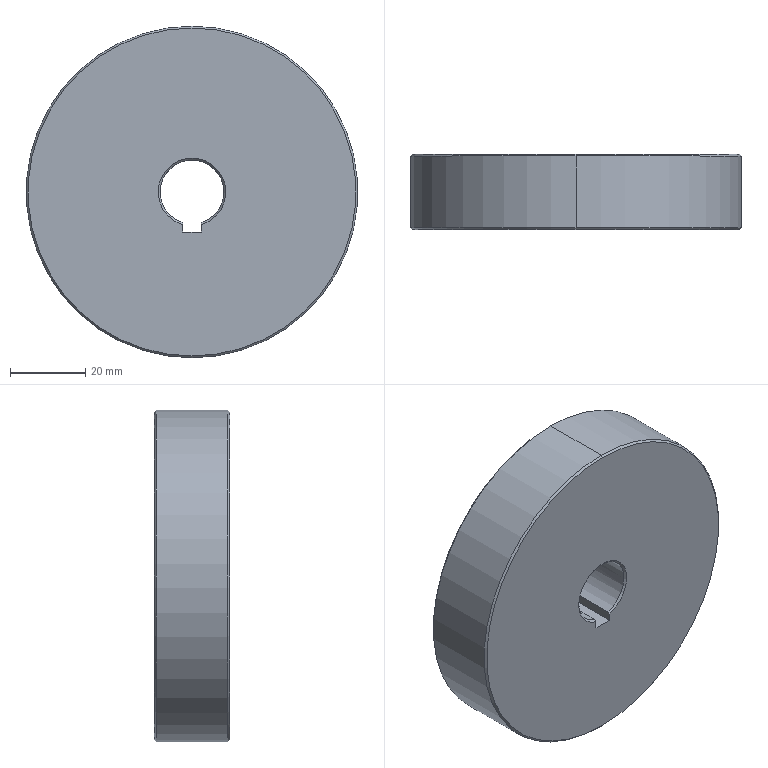Part | STEP file | Cuon T phu H01_6 | 1 solid | 15 faces | box 88 x 20 x 88 mm | volume 116797 mm3 | cone 7 | plane 5 | cylinder 3 | commonest cylinder face diameters 88 x2 17 x1
STEP:
#1=CARTESIAN_POINT('',(0.,0.,0.));
#2=DIRECTION('',(0.,0.,1.));
#3=DIRECTION('',(1.,0.,0.));
#4=AXIS2_PLACEMENT_3D('',#1,#2,#3);
#5=CARTESIAN_POINT('',(0.,20.,43.5));
#6=VERTEX_POINT('',#5);
#7=CARTESIAN_POINT('',(0.,20.,-43.5));
#8=VERTEX_POINT('',#7);
#9=CARTESIAN_POINT('',(0.,20.,0.));
#10=DIRECTION('',(0.,1.,0.));
#11=DIRECTION('',(0.,0.,1.));
#12=AXIS2_PLACEMENT_3D('',#9,#10,#11);
#13=CIRCLE('',#12,43.5);
#14=CARTESIAN_POINT('',(0.,20.,0.));
#15=DIRECTION('',(0.,-1.,0.));
#16=DIRECTION('',(0.,0.,-1.));
#17=AXIS2_PLACEMENT_3D('',#14,#15,#16);
#18=CONICAL_SURFACE('',#17,43.5,0.7854);
#19=CARTESIAN_POINT('',(3.142,0.));
#20=DIRECTION('',(-1.,0.));
#21=VECTOR('',#20,1.);
#22=LINE('',#19,#21);
#23=(GEOMETRIC_REPRESENTATION_CONTEXT(2)PARAMETRIC_REPRESENTATION_CONTEXT()REPRESENTATION_CONTEXT('',''));
#24=DEFINITIONAL_REPRESENTATION('',(#22),#23);
#25=PCURVE('',#18,#24);
#26=CARTESIAN_POINT('',(0.,20.,0.));
#27=DIRECTION('',(0.,1.,0.));
#28=DIRECTION('',(0.,0.,1.));
#29=AXIS2_PLACEMENT_3D('',#26,#27,#28);
#30=PLANE('',#29);
#31=CARTESIAN_POINT('',(0.,0.));
#32=DIRECTION('',(1.,0.));
#33=AXIS2_PLACEMENT_2D('',#31,#32);
#34=CIRCLE('',#33,43.5);
#35=(GEOMETRIC_REPRESENTATION_CONTEXT(2)PARAMETRIC_REPRESENTATION_CONTEXT()REPRESENTATION_CONTEXT('',''));
#36=DEFINITIONAL_REPRESENTATION('',(#34),#35);
#37=PCURVE('',#30,#36);
#38=SURFACE_CURVE('',#13,(#25,#37),.PCURVE_S1.);
#39=EDGE_CURVE('',#6,#8,#38,.T.);
#40=ORIENTED_EDGE('',*,*,#39,.F.);
#41=CARTESIAN_POINT('',(0.,19.5,44.));
#42=VERTEX_POINT('',#41);
#43=CARTESIAN_POINT('',(0.,20.,43.5));
#44=DIRECTION('',(0.,-0.7071,0.7071));
#45=VECTOR('',#44,1.);
#46=LINE('',#43,#45);
#47=CARTESIAN_POINT('',(3.142,0.));
#48=DIRECTION('',(0.,1.));
#49=VECTOR('',#48,1.);
#50=LINE('',#47,#49);
#51=(GEOMETRIC_REPRESENTATION_CONTEXT(2)PARAMETRIC_REPRESENTATION_CONTEXT()REPRESENTATION_CONTEXT('',''));
#52=DEFINITIONAL_REPRESENTATION('',(#50),#51);
#53=PCURVE('',#18,#52);
#54=CARTESIAN_POINT('',(0.,20.,0.));
#55=DIRECTION('',(0.,-1.,0.));
#56=DIRECTION('',(0.,0.,-1.));
#57=AXIS2_PLACEMENT_3D('',#54,#55,#56);
#58=CONICAL_SURFACE('',#57,43.5,0.7854);
#59=CARTESIAN_POINT('',(3.142,0.));
#60=DIRECTION('',(0.,1.));
#61=VECTOR('',#60,1.);
#62=LINE('',#59,#61);
#63=(GEOMETRIC_REPRESENTATION_CONTEXT(2)PARAMETRIC_REPRESENTATION_CONTEXT()REPRESENTATION_CONTEXT('',''));
#64=DEFINITIONAL_REPRESENTATION('',(#62),#63);
#65=PCURVE('',#58,#64);
#66=SURFACE_CURVE('',#46,(#53,#65),.PCURVE_S1.);
#67=EDGE_CURVE('',#6,#42,#66,.T.);
#68=ORIENTED_EDGE('',*,*,#67,.T.);
#69=CARTESIAN_POINT('',(0.,19.5,-44.));
#70=VERTEX_POINT('',#69);
#71=CARTESIAN_POINT('',(0.,19.5,0.));
#72=DIRECTION('',(0.,-1.,0.));
#73=DIRECTION('',(0.,0.,1.));
#74=AXIS2_PLACEMENT_3D('',#71,#72,#73);
#75=CIRCLE('',#74,44.);
#76=CARTESIAN_POINT('',(-3.142,0.5));
#77=DIRECTION('',(1.,0.));
#78=VECTOR('',#77,1.);
#79=LINE('',#76,#78);
#80=(GEOMETRIC_REPRESENTATION_CONTEXT(2)PARAMETRIC_REPRESENTATION_CONTEXT()REPRESENTATION_CONTEXT('',''));
#81=DEFINITIONAL_REPRESENTATION('',(#79),#80);
#82=PCURVE('',#18,#81);
#83=CARTESIAN_POINT('',(0.,20.,0.));
#84=DIRECTION('',(0.,-1.,0.));
#85=DIRECTION('',(0.,0.,-1.));
#86=AXIS2_PLACEMENT_3D('',#83,#84,#85);
#87=CYLINDRICAL_SURFACE('',#86,44.);
#88=CARTESIAN_POINT('',(-3.142,0.5));
#89=DIRECTION('',(1.,0.));
#90=VECTOR('',#89,1.);
#91=LINE('',#88,#90);
#92=(GEOMETRIC_REPRESENTATION_CONTEXT(2)PARAMETRIC_REPRESENTATION_CONTEXT()REPRESENTATION_CONTEXT('',''));
#93=DEFINITIONAL_REPRESENTATION('',(#91),#92);
#94=PCURVE('',#87,#93);
#95=SURFACE_CURVE('',#75,(#82,#94),.PCURVE_S1.);
#96=EDGE_CURVE('',#70,#42,#95,.T.);
#97=ORIENTED_EDGE('',*,*,#96,.F.);
#98=CARTESIAN_POINT('',(0.,20.,-43.5));
#99=DIRECTION('',(0.,-0.7071,-0.7071));
#100=VECTOR('',#99,1.);
#101=LINE('',#98,#100);
#102=CARTESIAN_POINT('',(0.,0.));
#103=DIRECTION('',(0.,1.));
#104=VECTOR('',#103,1.);
#105=LINE('',#102,#104);
#106=(GEOMETRIC_REPRESENTATION_CONTEXT(2)PARAMETRIC_REPRESENTATION_CONTEXT()REPRESENTATION_CONTEXT('',''));
#107=DEFINITIONAL_REPRESENTATION('',(#105),#106);
#108=PCURVE('',#18,#107);
#109=CARTESIAN_POINT('',(6.283,0.));
#110=DIRECTION('',(0.,1.));
#111=VECTOR('',#110,1.);
#112=LINE('',#109,#111);
#113=(GEOMETRIC_REPRESENTATION_CONTEXT(2)PARAMETRIC_REPRESENTATION_CONTEXT()REPRESENTATION_CONTEXT('',''));
#114=DEFINITIONAL_REPRESENTATION('',(#112),#113);
#115=PCURVE('',#58,#114);
#116=SURFACE_CURVE('',#101,(#108,#115),.PCURVE_S1.);
#117=EDGE_CURVE('',#8,#70,#116,.T.);
#118=ORIENTED_EDGE('',*,*,#117,.F.);
#119=EDGE_LOOP('',(#40,#68,#97,#118));
#120=FACE_BOUND('',#119,.T.);
#121=ADVANCED_FACE('',(#120),#18,.T.);
#122=CARTESIAN_POINT('',(0.,0.,-43.5));
#123=VERTEX_POINT('',#122);
#124=CARTESIAN_POINT('',(0.,0.,43.5));
#125=VERTEX_POINT('',#124);
#126=CARTESIAN_POINT('',(0.,0.,0.));
#127=DIRECTION('',(0.,-1.,0.));
#128=DIRECTION('',(0.,0.,1.));
#129=AXIS2_PLACEMENT_3D('',#126,#127,#128);
#130=CIRCLE('',#129,43.5);
#131=CARTESIAN_POINT('',(0.,0.5,0.));
#132=DIRECTION('',(0.,1.,0.));
#133=DIRECTION('',(0.,0.,1.));
#134=AXIS2_PLACEMENT_3D('',#131,#132,#133);
#135=CONICAL_SURFACE('',#134,44.,0.7854);
#136=CARTESIAN_POINT('',(6.283,-0.5));
#137=DIRECTION('',(-1.,0.));
#138=VECTOR('',#137,1.);
#139=LINE('',#136,#138);
#140=(GEOMETRIC_REPRESENTATION_CONTEXT(2)PARAMETRIC_REPRESENTATION_CONTEXT()REPRESENTATION_CONTEXT('',''));
#141=DEFINITIONAL_REPRESENTATION('',(#139),#140);
#142=PCURVE('',#135,#141);
#143=CARTESIAN_POINT('',(0.,0.,0.));
#144=DIRECTION('',(0.,1.,0.));
#145=DIRECTION('',(0.,0.,1.));
#146=AXIS2_PLACEMENT_3D('',#143,#144,#145);
#147=PLANE('',#146);
#148=CARTESIAN_POINT('',(43.5,0.));
#149=CARTESIAN_POINT('',(43.5,-75.344));
#150=CARTESIAN_POINT('',(-21.75,-37.672));
#151=CARTESIAN_POINT('',(-87.,0.));
#152=CARTESIAN_POINT('',(-21.75,37.672));
#153=CARTESIAN_POINT('',(43.5,75.344));
#154=CARTESIAN_POINT('',(43.5,0.));
#155=(BOUNDED_CURVE()B_SPLINE_CURVE(2,(#148,#149,#150,#151,#152,#153,#154),.UNSPECIFIED.,.T.,.F.)B_SPLINE_CURVE_WITH_KNOTS((1,2,2,2,2,1),(-2.094,0.,2.094,4.189,6.283,8.378),.UNSPECIFIED.)CURVE()GEOMETRIC_REPRESENTATION_ITEM()RATIONAL_B_SPLINE_CURVE((1.,0.5,1.,0.5,1.,0.5,1.))REPRESENTATION_ITEM(''));
#156=(GEOMETRIC_REPRESENTATION_CONTEXT(2)PARAMETRIC_REPRESENTATION_CONTEXT()REPRESENTATION_CONTEXT('',''));
#157=DEFINITIONAL_REPRESENTATION('',(#155),#156);
#158=PCURVE('',#147,#157);
#159=SURFACE_CURVE('',#130,(#142,#158),.PCURVE_S1.);
#160=EDGE_CURVE('',#123,#125,#159,.T.);
#161=ORIENTED_EDGE('',*,*,#160,.F.);
#162=CARTESIAN_POINT('',(0.,0.5,-44.));
#163=VERTEX_POINT('',#162);
#164=CARTESIAN_POINT('',(0.,0.5,-44.));
#165=DIRECTION('',(0.,0.7071,-0.7071));
#166=VECTOR('',#165,1.);
#167=LINE('',#164,#166);
#168=CARTESIAN_POINT('',(3.142,0.));
#169=DIRECTION('',(0.,1.));
#170=VECTOR('',#169,1.);
#171=LINE('',#168,#170);
#172=(GEOMETRIC_REPRESENTATION_CONTEXT(2)PARAMETRIC_REPRESENTATION_CONTEXT()REPRESENTATION_CONTEXT('',''));
#173=DEFINITIONAL_REPRESENTATION('',(#171),#172);
#174=PCURVE('',#135,#173);
#175=CARTESIAN_POINT('',(0.,0.5,0.));
#176=DIRECTION('',(0.,1.,0.));
#177=DIRECTION('',(0.,0.,1.));
#178=AXIS2_PLACEMENT_3D('',#175,#176,#177);
#179=CONICAL_SURFACE('',#178,44.,0.7854);
#180=CARTESIAN_POINT('',(3.142,0.));
#181=DIRECTION('',(0.,1.));
#182=VECTOR('',#181,1.);
#183=LINE('',#180,#182);
#184=(GEOMETRIC_REPRESENTATION_CONTEXT(2)PARAMETRIC_REPRESENTATION_CONTEXT()REPRESENTATION_CONTEXT('',''));
#185=DEFINITIONAL_REPRESENTATION('',(#183),#184);
#186=PCURVE('',#179,#185);
#187=SURFACE_CURVE('',#167,(#174,#186),.PCURVE_S1.);
#188=EDGE_CURVE('',#123,#163,#187,.T.);
#189=ORIENTED_EDGE('',*,*,#188,.T.);
#190=CARTESIAN_POINT('',(0.,0.5,44.));
#191=VERTEX_POINT('',#190);
#192=CARTESIAN_POINT('',(0.,0.5,0.));
#193=DIRECTION('',(0.,1.,0.));
#194=DIRECTION('',(0.,0.,1.));
#195=AXIS2_PLACEMENT_3D('',#192,#193,#194);
#196=CIRCLE('',#195,44.);
#197=CARTESIAN_POINT('',(0.,0.));
#198=DIRECTION('',(1.,0.));
#199=VECTOR('',#198,1.);
#200=LINE('',#197,#199);
#201=(GEOMETRIC_REPRESENTATION_CONTEXT(2)PARAMETRIC_REPRESENTATION_CONTEXT()REPRESENTATION_CONTEXT('',''));
#202=DEFINITIONAL_REPRESENTATION('',(#200),#201);
#203=PCURVE('',#135,#202);
#204=CARTESIAN_POINT('',(3.142,19.5));
#205=DIRECTION('',(-1.,0.));
#206=VECTOR('',#205,1.);
#207=LINE('',#204,#206);
#208=(GEOMETRIC_REPRESENTATION_CONTEXT(2)PARAMETRIC_REPRESENTATION_CONTEXT()REPRESENTATION_CONTEXT('',''));
#209=DEFINITIONAL_REPRESENTATION('',(#207),#208);
#210=PCURVE('',#87,#209);
#211=SURFACE_CURVE('',#196,(#203,#210),.PCURVE_S1.);
#212=EDGE_CURVE('',#191,#163,#211,.T.);
#213=ORIENTED_EDGE('',*,*,#212,.F.);
#214=CARTESIAN_POINT('',(0.,0.5,44.));
#215=DIRECTION('',(0.,0.7071,0.7071));
#216=VECTOR('',#215,1.);
#217=LINE('',#214,#216);
#218=CARTESIAN_POINT('',(0.,0.));
#219=DIRECTION('',(0.,1.));
#220=VECTOR('',#219,1.);
#221=LINE('',#218,#220);
#222=(GEOMETRIC_REPRESENTATION_CONTEXT(2)PARAMETRIC_REPRESENTATION_CONTEXT()REPRESENTATION_CONTEXT('',''));
#223=DEFINITIONAL_REPRESENTATION('',(#221),#222);
#224=PCURVE('',#135,#223);
#225=CARTESIAN_POINT('',(6.283,0.));
#226=DIRECTION('',(0.,1.));
#227=VECTOR('',#226,1.);
#228=LINE('',#225,#227);
#229=(GEOMETRIC_REPRESENTATION_CONTEXT(2)PARAMETRIC_REPRESENTATION_CONTEXT()REPRESENTATION_CONTEXT('',''));
#230=DEFINITIONAL_REPRESENTATION('',(#228),#229);
#231=PCURVE('',#179,#230);
#232=SURFACE_CURVE('',#217,(#224,#231),.PCURVE_S1.);
#233=EDGE_CURVE('',#125,#191,#232,.T.);
#234=ORIENTED_EDGE('',*,*,#233,.F.);
#235=EDGE_LOOP('',(#161,#189,#213,#234));
#236=FACE_BOUND('',#235,.T.);
#237=ADVANCED_FACE('',(#236),#135,.T.);
#238=CARTESIAN_POINT('',(2.5,19.5,-8.124));
#239=VERTEX_POINT('',#238);
#240=CARTESIAN_POINT('',(2.5,20.,-8.646));
#241=VERTEX_POINT('',#240);
#242=CARTESIAN_POINT('',(2.5,19.5,-8.124));
#243=CARTESIAN_POINT('',(2.5,19.666,-8.298));
#244=CARTESIAN_POINT('',(2.5,19.833,-8.472));
#245=CARTESIAN_POINT('',(2.5,20.,-8.646));
#246=B_SPLINE_CURVE_WITH_KNOTS('',3,(#242,#243,#244,#245),.UNSPECIFIED.,.F.,.F.,(4,4),(0.,0.0007227),.PIECEWISE_BEZIER_KNOTS.);
#247=CARTESIAN_POINT('',(0.,19.5,0.));
#248=DIRECTION('',(0.,1.,0.));
#249=DIRECTION('',(0.,0.,1.));
#250=AXIS2_PLACEMENT_3D('',#247,#248,#249);
#251=CONICAL_SURFACE('',#250,8.5,0.7854);
#252=CARTESIAN_POINT('',(2.843,0.));
#253=CARTESIAN_POINT('',(2.843,0.007565));
#254=CARTESIAN_POINT('',(2.844,0.0227));
#255=CARTESIAN_POINT('',(2.845,0.0454));
#256=CARTESIAN_POINT('',(2.846,0.0681));
#257=CARTESIAN_POINT('',(2.846,0.09081));
#258=CARTESIAN_POINT('',(2.847,0.1135));
#259=CARTESIAN_POINT('',(2.848,0.1362));
#260=CARTESIAN_POINT('',(2.849,0.1589));
#261=CARTESIAN_POINT('',(2.849,0.1817));
#262=CARTESIAN_POINT('',(2.85,0.2044));
#263=CARTESIAN_POINT('',(2.851,0.2271));
#264=CARTESIAN_POINT('',(2.852,0.2498));
#265=CARTESIAN_POINT('',(2.853,0.2726));
#266=CARTESIAN_POINT('',(2.853,0.2953));
#267=CARTESIAN_POINT('',(2.854,0.318));
#268=CARTESIAN_POINT('',(2.855,0.3408));
#269=CARTESIAN_POINT('',(2.856,0.3635));
#270=CARTESIAN_POINT('',(2.856,0.3862));
#271=CARTESIAN_POINT('',(2.857,0.409));
#272=CARTESIAN_POINT('',(2.858,0.4317));
#273=CARTESIAN_POINT('',(2.859,0.4545));
#274=CARTESIAN_POINT('',(2.859,0.4772));
#275=CARTESIAN_POINT('',(2.86,0.4924));
#276=CARTESIAN_POINT('',(2.86,0.5));
#277=B_SPLINE_CURVE_WITH_KNOTS('',3,(#252,#253,#254,#255,#256,#257,#258,#259,#260,#261,#262,#263,#264,#265,#266,#267,#268,#269,#270,#271,#272,#273,#274,#275,#276),.UNSPECIFIED.,.F.,.F.,(4,1,1,1,1,1,1,1,1,1,1,1,1,1,1,1,1,1,1,1,1,1,4),(0.,0.00003285,0.0000657,0.00009855,0.0001314,0.0001642,0.0001971,0.0002299,0.0002628,0.0002956,0.0003285,0.0003613,0.0003942,0.000427,0.0004599,0.0004927,0.0005256,0.0005584,0.0005913,0.0006241,0.000657,0.0006898,0.0007227),.QUASI_UNIFORM_KNOTS.);
#278=(GEOMETRIC_REPRESENTATION_CONTEXT(2)PARAMETRIC_REPRESENTATION_CONTEXT()REPRESENTATION_CONTEXT('',''));
#279=DEFINITIONAL_REPRESENTATION('',(#277),#278);
#280=PCURVE('',#251,#279);
#281=CARTESIAN_POINT('',(2.5,20.,-8.124));
#282=DIRECTION('',(-1.,0.,0.));
#283=DIRECTION('',(0.,0.,1.));
#284=AXIS2_PLACEMENT_3D('',#281,#282,#283);
#285=PLANE('',#284);
#286=CARTESIAN_POINT('',(0.,-0.5));
#287=CARTESIAN_POINT('',(-0.1741,-0.3336));
#288=CARTESIAN_POINT('',(-0.3481,-0.1669));
#289=CARTESIAN_POINT('',(-0.5218,0.));
#290=B_SPLINE_CURVE_WITH_KNOTS('',3,(#286,#287,#288,#289),.UNSPECIFIED.,.F.,.F.,(4,4),(0.,0.0007227),.PIECEWISE_BEZIER_KNOTS.);
#291=(GEOMETRIC_REPRESENTATION_CONTEXT(2)PARAMETRIC_REPRESENTATION_CONTEXT()REPRESENTATION_CONTEXT('',''));
#292=DEFINITIONAL_REPRESENTATION('',(#290),#291);
#293=PCURVE('',#285,#292);
#294=SURFACE_CURVE('',#246,(#280,#293),.PCURVE_S1.);
#295=EDGE_CURVE('',#239,#241,#294,.T.);
#296=ORIENTED_EDGE('',*,*,#295,.T.);
#297=CARTESIAN_POINT('',(0.,20.,9.));
#298=VERTEX_POINT('',#297);
#299=CARTESIAN_POINT('',(0.,20.,0.));
#300=DIRECTION('',(0.,-1.,0.));
#301=DIRECTION('',(0.,0.,1.));
#302=AXIS2_PLACEMENT_3D('',#299,#300,#301);
#303=CIRCLE('',#302,9.);
#304=CARTESIAN_POINT('',(6.283,0.5));
#305=DIRECTION('',(-1.,0.));
#306=VECTOR('',#305,1.);
#307=LINE('',#304,#306);
#308=(GEOMETRIC_REPRESENTATION_CONTEXT(2)PARAMETRIC_REPRESENTATION_CONTEXT()REPRESENTATION_CONTEXT('',''));
#309=DEFINITIONAL_REPRESENTATION('',(#307),#308);
#310=PCURVE('',#251,#309);
#311=CARTESIAN_POINT('',(9.,0.));
#312=CARTESIAN_POINT('',(9.,-15.588));
#313=CARTESIAN_POINT('',(-4.5,-7.794));
#314=CARTESIAN_POINT('',(-18.,0.));
#315=CARTESIAN_POINT('',(-4.5,7.794));
#316=CARTESIAN_POINT('',(9.,15.588));
#317=CARTESIAN_POINT('',(9.,0.));
#318=(BOUNDED_CURVE()B_SPLINE_CURVE(2,(#311,#312,#313,#314,#315,#316,#317),.UNSPECIFIED.,.T.,.F.)B_SPLINE_CURVE_WITH_KNOTS((1,2,2,2,2,1),(-2.094,0.,2.094,4.189,6.283,8.378),.UNSPECIFIED.)CURVE()GEOMETRIC_REPRESENTATION_ITEM()RATIONAL_B_SPLINE_CURVE((1.,0.5,1.,0.5,1.,0.5,1.))REPRESENTATION_ITEM(''));
#319=(GEOMETRIC_REPRESENTATION_CONTEXT(2)PARAMETRIC_REPRESENTATION_CONTEXT()REPRESENTATION_CONTEXT('',''));
#320=DEFINITIONAL_REPRESENTATION('',(#318),#319);
#321=PCURVE('',#30,#320);
#322=SURFACE_CURVE('',#303,(#310,#321),.PCURVE_S1.);
#323=EDGE_CURVE('',#241,#298,#322,.T.);
#324=ORIENTED_EDGE('',*,*,#323,.T.);
#325=CARTESIAN_POINT('',(0.,19.5,8.5));
#326=VERTEX_POINT('',#325);
#327=CARTESIAN_POINT('',(0.,19.5,8.5));
#328=DIRECTION('',(0.,0.7071,0.7071));
#329=VECTOR('',#328,1.);
#330=LINE('',#327,#329);
#331=CARTESIAN_POINT('',(0.,0.));
#332=DIRECTION('',(0.,1.));
#333=VECTOR('',#332,1.);
#334=LINE('',#331,#333);
#335=(GEOMETRIC_REPRESENTATION_CONTEXT(2)PARAMETRIC_REPRESENTATION_CONTEXT()REPRESENTATION_CONTEXT('',''));
#336=DEFINITIONAL_REPRESENTATION('',(#334),#335);
#337=PCURVE('',#251,#336);
#338=CARTESIAN_POINT('',(0.,19.5,0.));
#339=DIRECTION('',(0.,1.,0.));
#340=DIRECTION('',(0.,0.,1.));
#341=AXIS2_PLACEMENT_3D('',#338,#339,#340);
#342=CONICAL_SURFACE('',#341,8.5,0.7854);
#343=CARTESIAN_POINT('',(6.283,0.));
#344=DIRECTION('',(0.,1.));
#345=VECTOR('',#344,1.);
#346=LINE('',#343,#345);
#347=(GEOMETRIC_REPRESENTATION_CONTEXT(2)PARAMETRIC_REPRESENTATION_CONTEXT()REPRESENTATION_CONTEXT('',''));
#348=DEFINITIONAL_REPRESENTATION('',(#346),#347);
#349=PCURVE('',#342,#348);
#350=SURFACE_CURVE('',#330,(#337,#349),.PCURVE_S1.);
#351=EDGE_CURVE('',#326,#298,#350,.T.);
#352=ORIENTED_EDGE('',*,*,#351,.F.);
#353=CARTESIAN_POINT('',(0.,19.5,0.));
#354=DIRECTION('',(0.,1.,0.));
#355=DIRECTION('',(0.,0.,1.));
#356=AXIS2_PLACEMENT_3D('',#353,#354,#355);
#357=CIRCLE('',#356,8.5);
#358=CARTESIAN_POINT('',(0.,0.));
#359=DIRECTION('',(1.,0.));
#360=VECTOR('',#359,1.);
#361=LINE('',#358,#360);
#362=(GEOMETRIC_REPRESENTATION_CONTEXT(2)PARAMETRIC_REPRESENTATION_CONTEXT()REPRESENTATION_CONTEXT('',''));
#363=DEFINITIONAL_REPRESENTATION('',(#361),#362);
#364=PCURVE('',#251,#363);
#365=CARTESIAN_POINT('',(0.,20.,0.));
#366=DIRECTION('',(0.,-1.,0.));
#367=DIRECTION('',(0.,0.,-1.));
#368=AXIS2_PLACEMENT_3D('',#365,#366,#367);
#369=CYLINDRICAL_SURFACE('',#368,8.5);
#370=CARTESIAN_POINT('',(3.142,0.5));
#371=DIRECTION('',(-1.,0.));
#372=VECTOR('',#371,1.);
#373=LINE('',#370,#372);
#374=(GEOMETRIC_REPRESENTATION_CONTEXT(2)PARAMETRIC_REPRESENTATION_CONTEXT()REPRESENTATION_CONTEXT('',''));
#375=DEFINITIONAL_REPRESENTATION('',(#373),#374);
#376=PCURVE('',#369,#375);
#377=SURFACE_CURVE('',#357,(#364,#376),.PCURVE_S1.);
#378=EDGE_CURVE('',#326,#239,#377,.T.);
#379=ORIENTED_EDGE('',*,*,#378,.T.);
#380=EDGE_LOOP('',(#296,#324,#352,#379));
#381=FACE_BOUND('',#380,.F.);
#382=ADVANCED_FACE('',(#381),#251,.F.);
#383=ORIENTED_EDGE('',*,*,#96,.T.);
#384=CARTESIAN_POINT('',(0.,20.,44.));
#385=DIRECTION('',(0.,-1.,0.));
#386=VECTOR('',#385,1.);
#387=LINE('',#384,#386);
#388=CARTESIAN_POINT('',(3.142,0.));
#389=DIRECTION('',(0.,1.));
#390=VECTOR('',#389,1.);
#391=LINE('',#388,#390);
#392=(GEOMETRIC_REPRESENTATION_CONTEXT(2)PARAMETRIC_REPRESENTATION_CONTEXT()REPRESENTATION_CONTEXT('',''));
#393=DEFINITIONAL_REPRESENTATION('',(#391),#392);
#394=PCURVE('',#87,#393);
#395=CARTESIAN_POINT('',(0.,20.,0.));
#396=DIRECTION('',(0.,-1.,0.));
#397=DIRECTION('',(0.,0.,-1.));
#398=AXIS2_PLACEMENT_3D('',#395,#396,#397);
#399=CYLINDRICAL_SURFACE('',#398,44.);
#400=CARTESIAN_POINT('',(3.142,0.));
#401=DIRECTION('',(0.,1.));
#402=VECTOR('',#401,1.);
#403=LINE('',#400,#402);
#404=(GEOMETRIC_REPRESENTATION_CONTEXT(2)PARAMETRIC_REPRESENTATION_CONTEXT()REPRESENTATION_CONTEXT('',''));
#405=DEFINITIONAL_REPRESENTATION('',(#403),#404);
#406=PCURVE('',#399,#405);
#407=SURFACE_CURVE('',#387,(#394,#406),.PCURVE_S1.);
#408=EDGE_CURVE('',#42,#191,#407,.T.);
#409=ORIENTED_EDGE('',*,*,#408,.T.);
#410=ORIENTED_EDGE('',*,*,#212,.T.);
#411=CARTESIAN_POINT('',(0.,20.,-44.));
#412=DIRECTION('',(0.,-1.,0.));
#413=VECTOR('',#412,1.);
#414=LINE('',#411,#413);
#415=CARTESIAN_POINT('',(0.,0.));
#416=DIRECTION('',(0.,1.));
#417=VECTOR('',#416,1.);
#418=LINE('',#415,#417);
#419=(GEOMETRIC_REPRESENTATION_CONTEXT(2)PARAMETRIC_REPRESENTATION_CONTEXT()REPRESENTATION_CONTEXT('',''));
#420=DEFINITIONAL_REPRESENTATION('',(#418),#419);
#421=PCURVE('',#87,#420);
#422=CARTESIAN_POINT('',(6.283,0.));
#423=DIRECTION('',(0.,1.));
#424=VECTOR('',#423,1.);
#425=LINE('',#422,#424);
#426=(GEOMETRIC_REPRESENTATION_CONTEXT(2)PARAMETRIC_REPRESENTATION_CONTEXT()REPRESENTATION_CONTEXT('',''));
#427=DEFINITIONAL_REPRESENTATION('',(#425),#426);
#428=PCURVE('',#399,#427);
#429=SURFACE_CURVE('',#414,(#421,#428),.PCURVE_S1.);
#430=EDGE_CURVE('',#70,#163,#429,.T.);
#431=ORIENTED_EDGE('',*,*,#430,.F.);
#432=EDGE_LOOP('',(#383,#409,#410,#431));
#433=FACE_BOUND('',#432,.T.);
#434=ADVANCED_FACE('',(#433),#87,.T.);
#435=CARTESIAN_POINT('',(0.,20.,0.));
#436=DIRECTION('',(0.,1.,0.));
#437=DIRECTION('',(0.,0.,1.));
#438=AXIS2_PLACEMENT_3D('',#435,#436,#437);
#439=CIRCLE('',#438,43.5);
#440=CARTESIAN_POINT('',(0.,0.));
#441=DIRECTION('',(1.,0.));
#442=AXIS2_PLACEMENT_2D('',#440,#441);
#443=CIRCLE('',#442,43.5);
#444=(GEOMETRIC_REPRESENTATION_CONTEXT(2)PARAMETRIC_REPRESENTATION_CONTEXT()REPRESENTATION_CONTEXT('',''));
#445=DEFINITIONAL_REPRESENTATION('',(#443),#444);
#446=PCURVE('',#30,#445);
#447=CARTESIAN_POINT('',(9.425,0.));
#448=DIRECTION('',(-1.,0.));
#449=VECTOR('',#448,1.);
#450=LINE('',#447,#449);
#451=(GEOMETRIC_REPRESENTATION_CONTEXT(2)PARAMETRIC_REPRESENTATION_CONTEXT()REPRESENTATION_CONTEXT('',''));
#452=DEFINITIONAL_REPRESENTATION('',(#450),#451);
#453=PCURVE('',#58,#452);
#454=SURFACE_CURVE('',#439,(#446,#453),.PCURVE_S1.);
#455=EDGE_CURVE('',#8,#6,#454,.T.);
#456=ORIENTED_EDGE('',*,*,#455,.T.);
#457=ORIENTED_EDGE('',*,*,#39,.T.);
#458=EDGE_LOOP('',(#456,#457));
#459=FACE_BOUND('',#458,.T.);
#460=CARTESIAN_POINT('',(2.5,20.,-10.624));
#461=VERTEX_POINT('',#460);
#462=CARTESIAN_POINT('',(2.5,20.,-8.124));
#463=DIRECTION('',(0.,0.,-1.));
#464=VECTOR('',#463,1.);
#465=LINE('',#462,#464);
#466=CARTESIAN_POINT('',(-8.124,2.5));
#467=DIRECTION('',(-1.,0.));
#468=VECTOR('',#467,1.);
#469=LINE('',#466,#468);
#470=(GEOMETRIC_REPRESENTATION_CONTEXT(2)PARAMETRIC_REPRESENTATION_CONTEXT()REPRESENTATION_CONTEXT('',''));
#471=DEFINITIONAL_REPRESENTATION('',(#469),#470);
#472=PCURVE('',#30,#471);
#473=CARTESIAN_POINT('',(0.,0.));
#474=DIRECTION('',(-1.,0.));
#475=VECTOR('',#474,1.);
#476=LINE('',#473,#475);
#477=(GEOMETRIC_REPRESENTATION_CONTEXT(2)PARAMETRIC_REPRESENTATION_CONTEXT()REPRESENTATION_CONTEXT('',''));
#478=DEFINITIONAL_REPRESENTATION('',(#476),#477);
#479=PCURVE('',#285,#478);
#480=SURFACE_CURVE('',#465,(#472,#479),.PCURVE_S1.);
#481=EDGE_CURVE('',#241,#461,#480,.T.);
#482=ORIENTED_EDGE('',*,*,#481,.F.);
#483=ORIENTED_EDGE('',*,*,#323,.T.);
#484=CARTESIAN_POINT('',(-2.5,20.,-8.646));
#485=VERTEX_POINT('',#484);
#486=CARTESIAN_POINT('',(0.,20.,0.));
#487=DIRECTION('',(0.,-1.,0.));
#488=DIRECTION('',(0.,0.,1.));
#489=AXIS2_PLACEMENT_3D('',#486,#487,#488);
#490=CIRCLE('',#489,9.);
#491=CARTESIAN_POINT('',(9.,0.));
#492=CARTESIAN_POINT('',(9.,-15.588));
#493=CARTESIAN_POINT('',(-4.5,-7.794));
#494=CARTESIAN_POINT('',(-18.,0.));
#495=CARTESIAN_POINT('',(-4.5,7.794));
#496=CARTESIAN_POINT('',(9.,15.588));
#497=CARTESIAN_POINT('',(9.,0.));
#498=(BOUNDED_CURVE()B_SPLINE_CURVE(2,(#491,#492,#493,#494,#495,#496,#497),.UNSPECIFIED.,.T.,.F.)B_SPLINE_CURVE_WITH_KNOTS((1,2,2,2,2,1),(-2.094,0.,2.094,4.189,6.283,8.378),.UNSPECIFIED.)CURVE()GEOMETRIC_REPRESENTATION_ITEM()RATIONAL_B_SPLINE_CURVE((1.,0.5,1.,0.5,1.,0.5,1.))REPRESENTATION_ITEM(''));
#499=(GEOMETRIC_REPRESENTATION_CONTEXT(2)PARAMETRIC_REPRESENTATION_CONTEXT()REPRESENTATION_CONTEXT('',''));
#500=DEFINITIONAL_REPRESENTATION('',(#498),#499);
#501=PCURVE('',#30,#500);
#502=CARTESIAN_POINT('',(6.283,0.5));
#503=DIRECTION('',(-1.,0.));
#504=VECTOR('',#503,1.);
#505=LINE('',#502,#504);
#506=(GEOMETRIC_REPRESENTATION_CONTEXT(2)PARAMETRIC_REPRESENTATION_CONTEXT()REPRESENTATION_CONTEXT('',''));
#507=DEFINITIONAL_REPRESENTATION('',(#505),#506);
#508=PCURVE('',#342,#507);
#509=SURFACE_CURVE('',#490,(#501,#508),.PCURVE_S1.);
#510=EDGE_CURVE('',#298,#485,#509,.T.);
#511=ORIENTED_EDGE('',*,*,#510,.T.);
#512=CARTESIAN_POINT('',(-2.5,20.,-10.624));
#513=VERTEX_POINT('',#512);
#514=CARTESIAN_POINT('',(-2.5,20.,-8.124));
#515=DIRECTION('',(0.,0.,1.));
#516=VECTOR('',#515,1.);
#517=LINE('',#514,#516);
#518=CARTESIAN_POINT('',(-8.124,-2.5));
#519=DIRECTION('',(1.,0.));
#520=VECTOR('',#519,1.);
#521=LINE('',#518,#520);
#522=(GEOMETRIC_REPRESENTATION_CONTEXT(2)PARAMETRIC_REPRESENTATION_CONTEXT()REPRESENTATION_CONTEXT('',''));
#523=DEFINITIONAL_REPRESENTATION('',(#521),#522);
#524=PCURVE('',#30,#523);
#525=CARTESIAN_POINT('',(-2.5,20.,-8.124));
#526=DIRECTION('',(1.,0.,0.));
#527=DIRECTION('',(0.,0.,-1.));
#528=AXIS2_PLACEMENT_3D('',#525,#526,#527);
#529=PLANE('',#528);
#530=CARTESIAN_POINT('',(0.,0.));
#531=DIRECTION('',(-1.,0.));
#532=VECTOR('',#531,1.);
#533=LINE('',#530,#532);
#534=(GEOMETRIC_REPRESENTATION_CONTEXT(2)PARAMETRIC_REPRESENTATION_CONTEXT()REPRESENTATION_CONTEXT('',''));
#535=DEFINITIONAL_REPRESENTATION('',(#533),#534);
#536=PCURVE('',#529,#535);
#537=SURFACE_CURVE('',#517,(#524,#536),.PCURVE_S1.);
#538=EDGE_CURVE('',#513,#485,#537,.T.);
#539=ORIENTED_EDGE('',*,*,#538,.F.);
#540=CARTESIAN_POINT('',(-2.5,20.,-10.624));
#541=DIRECTION('',(-1.,0.,0.));
#542=VECTOR('',#541,1.);
#543=LINE('',#540,#542);
#544=CARTESIAN_POINT('',(-10.624,-2.5));
#545=DIRECTION('',(0.,-1.));
#546=VECTOR('',#545,1.);
#547=LINE('',#544,#546);
#548=(GEOMETRIC_REPRESENTATION_CONTEXT(2)PARAMETRIC_REPRESENTATION_CONTEXT()REPRESENTATION_CONTEXT('',''));
#549=DEFINITIONAL_REPRESENTATION('',(#547),#548);
#550=PCURVE('',#30,#549);
#551=CARTESIAN_POINT('',(-2.5,20.,-10.624));
#552=DIRECTION('',(0.,0.,1.));
#553=DIRECTION('',(1.,0.,0.));
#554=AXIS2_PLACEMENT_3D('',#551,#552,#553);
#555=PLANE('',#554);
#556=CARTESIAN_POINT('',(0.,0.));
#557=DIRECTION('',(-1.,0.));
#558=VECTOR('',#557,1.);
#559=LINE('',#556,#558);
#560=(GEOMETRIC_REPRESENTATION_CONTEXT(2)PARAMETRIC_REPRESENTATION_CONTEXT()REPRESENTATION_CONTEXT('',''));
#561=DEFINITIONAL_REPRESENTATION('',(#559),#560);
#562=PCURVE('',#555,#561);
#563=SURFACE_CURVE('',#543,(#550,#562),.PCURVE_S1.);
#564=EDGE_CURVE('',#461,#513,#563,.T.);
#565=ORIENTED_EDGE('',*,*,#564,.F.);
#566=EDGE_LOOP('',(#482,#483,#511,#539,#565));
#567=FACE_BOUND('',#566,.T.);
#568=ADVANCED_FACE('',(#459,#567),#30,.T.);
#569=CARTESIAN_POINT('',(0.,0.,0.));
#570=DIRECTION('',(0.,-1.,0.));
#571=DIRECTION('',(0.,0.,1.));
#572=AXIS2_PLACEMENT_3D('',#569,#570,#571);
#573=CIRCLE('',#572,43.5);
#574=CARTESIAN_POINT('',(43.5,0.));
#575=CARTESIAN_POINT('',(43.5,-75.344));
#576=CARTESIAN_POINT('',(-21.75,-37.672));
#577=CARTESIAN_POINT('',(-87.,0.));
#578=CARTESIAN_POINT('',(-21.75,37.672));
#579=CARTESIAN_POINT('',(43.5,75.344));
#580=CARTESIAN_POINT('',(43.5,0.));
#581=(BOUNDED_CURVE()B_SPLINE_CURVE(2,(#574,#575,#576,#577,#578,#579,#580),.UNSPECIFIED.,.T.,.F.)B_SPLINE_CURVE_WITH_KNOTS((1,2,2,2,2,1),(-2.094,0.,2.094,4.189,6.283,8.378),.UNSPECIFIED.)CURVE()GEOMETRIC_REPRESENTATION_ITEM()RATIONAL_B_SPLINE_CURVE((1.,0.5,1.,0.5,1.,0.5,1.))REPRESENTATION_ITEM(''));
#582=(GEOMETRIC_REPRESENTATION_CONTEXT(2)PARAMETRIC_REPRESENTATION_CONTEXT()REPRESENTATION_CONTEXT('',''));
#583=DEFINITIONAL_REPRESENTATION('',(#581),#582);
#584=PCURVE('',#147,#583);
#585=CARTESIAN_POINT('',(6.283,-0.5));
#586=DIRECTION('',(-1.,0.));
#587=VECTOR('',#586,1.);
#588=LINE('',#585,#587);
#589=(GEOMETRIC_REPRESENTATION_CONTEXT(2)PARAMETRIC_REPRESENTATION_CONTEXT()REPRESENTATION_CONTEXT('',''));
#590=DEFINITIONAL_REPRESENTATION('',(#588),#589);
#591=PCURVE('',#179,#590);
#592=SURFACE_CURVE('',#573,(#584,#591),.PCURVE_S1.);
#593=EDGE_CURVE('',#125,#123,#592,.T.);
#594=ORIENTED_EDGE('',*,*,#593,.T.);
#595=ORIENTED_EDGE('',*,*,#160,.T.);
#596=EDGE_LOOP('',(#594,#595));
#597=FACE_BOUND('',#596,.T.);
#598=CARTESIAN_POINT('',(-2.5,0.,-10.624));
#599=VERTEX_POINT('',#598);
#600=CARTESIAN_POINT('',(-2.5,0.,-8.646));
#601=VERTEX_POINT('',#600);
#602=CARTESIAN_POINT('',(-2.5,0.,-8.124));
#603=DIRECTION('',(0.,0.,1.));
#604=VECTOR('',#603,1.);
#605=LINE('',#602,#604);
#606=CARTESIAN_POINT('',(-8.124,-2.5));
#607=DIRECTION('',(1.,0.));
#608=VECTOR('',#607,1.);
#609=LINE('',#606,#608);
#610=(GEOMETRIC_REPRESENTATION_CONTEXT(2)PARAMETRIC_REPRESENTATION_CONTEXT()REPRESENTATION_CONTEXT('',''));
#611=DEFINITIONAL_REPRESENTATION('',(#609),#610);
#612=PCURVE('',#147,#611);
#613=CARTESIAN_POINT('',(0.,-20.));
#614=DIRECTION('',(-1.,0.));
#615=VECTOR('',#614,1.);
#616=LINE('',#613,#615);
#617=(GEOMETRIC_REPRESENTATION_CONTEXT(2)PARAMETRIC_REPRESENTATION_CONTEXT()REPRESENTATION_CONTEXT('',''));
#618=DEFINITIONAL_REPRESENTATION('',(#616),#617);
#619=PCURVE('',#529,#618);
#620=SURFACE_CURVE('',#605,(#612,#619),.PCURVE_S1.);
#621=EDGE_CURVE('',#599,#601,#620,.T.);
#622=ORIENTED_EDGE('',*,*,#621,.T.);
#623=CARTESIAN_POINT('',(2.5,0.,-8.646));
#624=VERTEX_POINT('',#623);
#625=CARTESIAN_POINT('',(0.,0.,0.));
#626=DIRECTION('',(0.,1.,0.));
#627=DIRECTION('',(0.,0.,1.));
#628=AXIS2_PLACEMENT_3D('',#625,#626,#627);
#629=CIRCLE('',#628,9.);
#630=CARTESIAN_POINT('',(0.,0.));
#631=DIRECTION('',(1.,0.));
#632=AXIS2_PLACEMENT_2D('',#630,#631);
#633=CIRCLE('',#632,9.);
#634=(GEOMETRIC_REPRESENTATION_CONTEXT(2)PARAMETRIC_REPRESENTATION_CONTEXT()REPRESENTATION_CONTEXT('',''));
#635=DEFINITIONAL_REPRESENTATION('',(#633),#634);
#636=PCURVE('',#147,#635);
#637=CARTESIAN_POINT('',(0.,0.,0.));
#638=DIRECTION('',(0.,-1.,0.));
#639=DIRECTION('',(0.,0.,-1.));
#640=AXIS2_PLACEMENT_3D('',#637,#638,#639);
#641=CONICAL_SURFACE('',#640,9.,0.7854);
#642=CARTESIAN_POINT('',(9.425,0.));
#643=DIRECTION('',(-1.,0.));
#644=VECTOR('',#643,1.);
#645=LINE('',#642,#644);
#646=(GEOMETRIC_REPRESENTATION_CONTEXT(2)PARAMETRIC_REPRESENTATION_CONTEXT()REPRESENTATION_CONTEXT('',''));
#647=DEFINITIONAL_REPRESENTATION('',(#645),#646);
#648=PCURVE('',#641,#647);
#649=SURFACE_CURVE('',#629,(#636,#648),.PCURVE_S1.);
#650=EDGE_CURVE('',#601,#624,#649,.T.);
#651=ORIENTED_EDGE('',*,*,#650,.T.);
#652=CARTESIAN_POINT('',(2.5,0.,-10.624));
#653=VERTEX_POINT('',#652);
#654=CARTESIAN_POINT('',(2.5,0.,-8.124));
#655=DIRECTION('',(0.,0.,-1.));
#656=VECTOR('',#655,1.);
#657=LINE('',#654,#656);
#658=CARTESIAN_POINT('',(-8.124,2.5));
#659=DIRECTION('',(-1.,0.));
#660=VECTOR('',#659,1.);
#661=LINE('',#658,#660);
#662=(GEOMETRIC_REPRESENTATION_CONTEXT(2)PARAMETRIC_REPRESENTATION_CONTEXT()REPRESENTATION_CONTEXT('',''));
#663=DEFINITIONAL_REPRESENTATION('',(#661),#662);
#664=PCURVE('',#147,#663);
#665=CARTESIAN_POINT('',(0.,-20.));
#666=DIRECTION('',(-1.,0.));
#667=VECTOR('',#666,1.);
#668=LINE('',#665,#667);
#669=(GEOMETRIC_REPRESENTATION_CONTEXT(2)PARAMETRIC_REPRESENTATION_CONTEXT()REPRESENTATION_CONTEXT('',''));
#670=DEFINITIONAL_REPRESENTATION('',(#668),#669);
#671=PCURVE('',#285,#670);
#672=SURFACE_CURVE('',#657,(#664,#671),.PCURVE_S1.);
#673=EDGE_CURVE('',#624,#653,#672,.T.);
#674=ORIENTED_EDGE('',*,*,#673,.T.);
#675=CARTESIAN_POINT('',(-2.5,0.,-10.624));
#676=DIRECTION('',(-1.,0.,0.));
#677=VECTOR('',#676,1.);
#678=LINE('',#675,#677);
#679=CARTESIAN_POINT('',(-10.624,-2.5));
#680=DIRECTION('',(0.,-1.));
#681=VECTOR('',#680,1.);
#682=LINE('',#679,#681);
#683=(GEOMETRIC_REPRESENTATION_CONTEXT(2)PARAMETRIC_REPRESENTATION_CONTEXT()REPRESENTATION_CONTEXT('',''));
#684=DEFINITIONAL_REPRESENTATION('',(#682),#683);
#685=PCURVE('',#147,#684);
#686=CARTESIAN_POINT('',(0.,-20.));
#687=DIRECTION('',(-1.,0.));
#688=VECTOR('',#687,1.);
#689=LINE('',#686,#688);
#690=(GEOMETRIC_REPRESENTATION_CONTEXT(2)PARAMETRIC_REPRESENTATION_CONTEXT()REPRESENTATION_CONTEXT('',''));
#691=DEFINITIONAL_REPRESENTATION('',(#689),#690);
#692=PCURVE('',#555,#691);
#693=SURFACE_CURVE('',#678,(#685,#692),.PCURVE_S1.);
#694=EDGE_CURVE('',#653,#599,#693,.T.);
#695=ORIENTED_EDGE('',*,*,#694,.T.);
#696=EDGE_LOOP('',(#622,#651,#674,#695));
#697=FACE_BOUND('',#696,.T.);
#698=ADVANCED_FACE('',(#597,#697),#147,.F.);
#699=ORIENTED_EDGE('',*,*,#408,.F.);
#700=CARTESIAN_POINT('',(0.,19.5,0.));
#701=DIRECTION('',(0.,-1.,0.));
#702=DIRECTION('',(0.,0.,1.));
#703=AXIS2_PLACEMENT_3D('',#700,#701,#702);
#704=CIRCLE('',#703,44.);
#705=CARTESIAN_POINT('',(3.142,0.5));
#706=DIRECTION('',(1.,0.));
#707=VECTOR('',#706,1.);
#708=LINE('',#705,#707);
#709=(GEOMETRIC_REPRESENTATION_CONTEXT(2)PARAMETRIC_REPRESENTATION_CONTEXT()REPRESENTATION_CONTEXT('',''));
#710=DEFINITIONAL_REPRESENTATION('',(#708),#709);
#711=PCURVE('',#399,#710);
#712=CARTESIAN_POINT('',(3.142,0.5));
#713=DIRECTION('',(1.,0.));
#714=VECTOR('',#713,1.);
#715=LINE('',#712,#714);
#716=(GEOMETRIC_REPRESENTATION_CONTEXT(2)PARAMETRIC_REPRESENTATION_CONTEXT()REPRESENTATION_CONTEXT('',''));
#717=DEFINITIONAL_REPRESENTATION('',(#715),#716);
#718=PCURVE('',#58,#717);
#719=SURFACE_CURVE('',#704,(#711,#718),.PCURVE_S1.);
#720=EDGE_CURVE('',#42,#70,#719,.T.);
#721=ORIENTED_EDGE('',*,*,#720,.T.);
#722=ORIENTED_EDGE('',*,*,#430,.T.);
#723=CARTESIAN_POINT('',(0.,0.5,0.));
#724=DIRECTION('',(0.,1.,0.));
#725=DIRECTION('',(0.,0.,1.));
#726=AXIS2_PLACEMENT_3D('',#723,#724,#725);
#727=CIRCLE('',#726,44.);
#728=CARTESIAN_POINT('',(9.425,19.5));
#729=DIRECTION('',(-1.,0.));
#730=VECTOR('',#729,1.);
#731=LINE('',#728,#730);
#732=(GEOMETRIC_REPRESENTATION_CONTEXT(2)PARAMETRIC_REPRESENTATION_CONTEXT()REPRESENTATION_CONTEXT('',''));
#733=DEFINITIONAL_REPRESENTATION('',(#731),#732);
#734=PCURVE('',#399,#733);
#735=CARTESIAN_POINT('',(0.,0.));
#736=DIRECTION('',(1.,0.));
#737=VECTOR('',#736,1.);
#738=LINE('',#735,#737);
#739=(GEOMETRIC_REPRESENTATION_CONTEXT(2)PARAMETRIC_REPRESENTATION_CONTEXT()REPRESENTATION_CONTEXT('',''));
#740=DEFINITIONAL_REPRESENTATION('',(#738),#739);
#741=PCURVE('',#179,#740);
#742=SURFACE_CURVE('',#727,(#734,#741),.PCURVE_S1.);
#743=EDGE_CURVE('',#163,#191,#742,.T.);
#744=ORIENTED_EDGE('',*,*,#743,.T.);
#745=EDGE_LOOP('',(#699,#721,#722,#744));
#746=FACE_BOUND('',#745,.T.);
#747=ADVANCED_FACE('',(#746),#399,.T.);
#748=ORIENTED_EDGE('',*,*,#673,.F.);
#749=CARTESIAN_POINT('',(2.5,0.5,-8.124));
#750=VERTEX_POINT('',#749);
#751=CARTESIAN_POINT('',(2.5,0.,-8.646));
#752=CARTESIAN_POINT('',(2.5,0.1669,-8.472));
#753=CARTESIAN_POINT('',(2.5,0.3336,-8.298));
#754=CARTESIAN_POINT('',(2.5,0.5,-8.124));
#755=B_SPLINE_CURVE_WITH_KNOTS('',3,(#751,#752,#753,#754),.UNSPECIFIED.,.F.,.F.,(4,4),(0.,0.0007227),.PIECEWISE_BEZIER_KNOTS.);
#756=CARTESIAN_POINT('',(-0.5218,-20.));
#757=CARTESIAN_POINT('',(-0.3481,-19.833));
#758=CARTESIAN_POINT('',(-0.1741,-19.666));
#759=CARTESIAN_POINT('',(0.,-19.5));
#760=B_SPLINE_CURVE_WITH_KNOTS('',3,(#756,#757,#758,#759),.UNSPECIFIED.,.F.,.F.,(4,4),(0.,0.0007227),.PIECEWISE_BEZIER_KNOTS.);
#761=(GEOMETRIC_REPRESENTATION_CONTEXT(2)PARAMETRIC_REPRESENTATION_CONTEXT()REPRESENTATION_CONTEXT('',''));
#762=DEFINITIONAL_REPRESENTATION('',(#760),#761);
#763=PCURVE('',#285,#762);
#764=CARTESIAN_POINT('',(0.2815,0.));
#765=CARTESIAN_POINT('',(0.2817,-0.007586));
#766=CARTESIAN_POINT('',(0.2822,-0.02276));
#767=CARTESIAN_POINT('',(0.2829,-0.04551));
#768=CARTESIAN_POINT('',(0.2837,-0.06826));
#769=CARTESIAN_POINT('',(0.2844,-0.09101));
#770=CARTESIAN_POINT('',(0.2852,-0.1138));
#771=CARTESIAN_POINT('',(0.2859,-0.1365));
#772=CARTESIAN_POINT('',(0.2867,-0.1592));
#773=CARTESIAN_POINT('',(0.2875,-0.182));
#774=CARTESIAN_POINT('',(0.2882,-0.2047));
#775=CARTESIAN_POINT('',(0.289,-0.2274));
#776=CARTESIAN_POINT('',(0.2898,-0.2502));
#777=CARTESIAN_POINT('',(0.2905,-0.2729));
#778=CARTESIAN_POINT('',(0.2913,-0.2956));
#779=CARTESIAN_POINT('',(0.2921,-0.3183));
#780=CARTESIAN_POINT('',(0.2929,-0.3411));
#781=CARTESIAN_POINT('',(0.2937,-0.3638));
#782=CARTESIAN_POINT('',(0.2945,-0.3865));
#783=CARTESIAN_POINT('',(0.2953,-0.4092));
#784=CARTESIAN_POINT('',(0.2961,-0.4319));
#785=CARTESIAN_POINT('',(0.2969,-0.4546));
#786=CARTESIAN_POINT('',(0.2977,-0.4773));
#787=CARTESIAN_POINT('',(0.2983,-0.4924));
#788=CARTESIAN_POINT('',(0.2985,-0.5));
#789=B_SPLINE_CURVE_WITH_KNOTS('',3,(#764,#765,#766,#767,#768,#769,#770,#771,#772,#773,#774,#775,#776,#777,#778,#779,#780,#781,#782,#783,#784,#785,#786,#787,#788),.UNSPECIFIED.,.F.,.F.,(4,1,1,1,1,1,1,1,1,1,1,1,1,1,1,1,1,1,1,1,1,1,4),(0.,0.00003285,0.0000657,0.00009855,0.0001314,0.0001642,0.0001971,0.0002299,0.0002628,0.0002956,0.0003285,0.0003613,0.0003942,0.000427,0.0004599,0.0004927,0.0005256,0.0005584,0.0005913,0.0006241,0.000657,0.0006898,0.0007227),.QUASI_UNIFORM_KNOTS.);
#790=(GEOMETRIC_REPRESENTATION_CONTEXT(2)PARAMETRIC_REPRESENTATION_CONTEXT()REPRESENTATION_CONTEXT('',''));
#791=DEFINITIONAL_REPRESENTATION('',(#789),#790);
#792=PCURVE('',#641,#791);
#793=SURFACE_CURVE('',#755,(#763,#792),.PCURVE_S1.);
#794=EDGE_CURVE('',#624,#750,#793,.T.);
#795=ORIENTED_EDGE('',*,*,#794,.T.);
#796=CARTESIAN_POINT('',(2.5,20.,-8.124));
#797=DIRECTION('',(0.,-1.,0.));
#798=VECTOR('',#797,1.);
#799=LINE('',#796,#798);
#800=CARTESIAN_POINT('',(0.,0.));
#801=DIRECTION('',(0.,-1.));
#802=VECTOR('',#801,1.);
#803=LINE('',#800,#802);
#804=(GEOMETRIC_REPRESENTATION_CONTEXT(2)PARAMETRIC_REPRESENTATION_CONTEXT()REPRESENTATION_CONTEXT('',''));
#805=DEFINITIONAL_REPRESENTATION('',(#803),#804);
#806=PCURVE('',#285,#805);
#807=CARTESIAN_POINT('',(0.2985,0.));
#808=DIRECTION('',(0.,1.));
#809=VECTOR('',#808,1.);
#810=LINE('',#807,#809);
#811=(GEOMETRIC_REPRESENTATION_CONTEXT(2)PARAMETRIC_REPRESENTATION_CONTEXT()REPRESENTATION_CONTEXT('',''));
#812=DEFINITIONAL_REPRESENTATION('',(#810),#811);
#813=PCURVE('',#369,#812);
#814=SURFACE_CURVE('',#799,(#806,#813),.PCURVE_S1.);
#815=EDGE_CURVE('',#239,#750,#814,.T.);
#816=ORIENTED_EDGE('',*,*,#815,.F.);
#817=ORIENTED_EDGE('',*,*,#295,.T.);
#818=ORIENTED_EDGE('',*,*,#481,.T.);
#819=CARTESIAN_POINT('',(2.5,20.,-10.624));
#820=DIRECTION('',(0.,-1.,0.));
#821=VECTOR('',#820,1.);
#822=LINE('',#819,#821);
#823=CARTESIAN_POINT('',(-2.5,0.));
#824=DIRECTION('',(0.,-1.));
#825=VECTOR('',#824,1.);
#826=LINE('',#823,#825);
#827=(GEOMETRIC_REPRESENTATION_CONTEXT(2)PARAMETRIC_REPRESENTATION_CONTEXT()REPRESENTATION_CONTEXT('',''));
#828=DEFINITIONAL_REPRESENTATION('',(#826),#827);
#829=PCURVE('',#285,#828);
#830=CARTESIAN_POINT('',(5.,0.));
#831=DIRECTION('',(0.,-1.));
#832=VECTOR('',#831,1.);
#833=LINE('',#830,#832);
#834=(GEOMETRIC_REPRESENTATION_CONTEXT(2)PARAMETRIC_REPRESENTATION_CONTEXT()REPRESENTATION_CONTEXT('',''));
#835=DEFINITIONAL_REPRESENTATION('',(#833),#834);
#836=PCURVE('',#555,#835);
#837=SURFACE_CURVE('',#822,(#829,#836),.PCURVE_S1.);
#838=EDGE_CURVE('',#461,#653,#837,.T.);
#839=ORIENTED_EDGE('',*,*,#838,.T.);
#840=EDGE_LOOP('',(#748,#795,#816,#817,#818,#839));
#841=FACE_BOUND('',#840,.T.);
#842=ADVANCED_FACE('',(#841),#285,.T.);
#843=ORIENTED_EDGE('',*,*,#694,.F.);
#844=ORIENTED_EDGE('',*,*,#838,.F.);
#845=ORIENTED_EDGE('',*,*,#564,.T.);
#846=CARTESIAN_POINT('',(-2.5,20.,-10.624));
#847=DIRECTION('',(0.,-1.,0.));
#848=VECTOR('',#847,1.);
#849=LINE('',#846,#848);
#850=CARTESIAN_POINT('',(0.,0.));
#851=DIRECTION('',(0.,-1.));
#852=VECTOR('',#851,1.);
#853=LINE('',#850,#852);
#854=(GEOMETRIC_REPRESENTATION_CONTEXT(2)PARAMETRIC_REPRESENTATION_CONTEXT()REPRESENTATION_CONTEXT('',''));
#855=DEFINITIONAL_REPRESENTATION('',(#853),#854);
#856=PCURVE('',#555,#855);
#857=CARTESIAN_POINT('',(2.5,0.));
#858=DIRECTION('',(0.,-1.));
#859=VECTOR('',#858,1.);
#860=LINE('',#857,#859);
#861=(GEOMETRIC_REPRESENTATION_CONTEXT(2)PARAMETRIC_REPRESENTATION_CONTEXT()REPRESENTATION_CONTEXT('',''));
#862=DEFINITIONAL_REPRESENTATION('',(#860),#861);
#863=PCURVE('',#529,#862);
#864=SURFACE_CURVE('',#849,(#856,#863),.PCURVE_S1.);
#865=EDGE_CURVE('',#513,#599,#864,.T.);
#866=ORIENTED_EDGE('',*,*,#865,.T.);
#867=EDGE_LOOP('',(#843,#844,#845,#866));
#868=FACE_BOUND('',#867,.T.);
#869=ADVANCED_FACE('',(#868),#555,.T.);
#870=CARTESIAN_POINT('',(-2.5,19.5,-8.124));
#871=VERTEX_POINT('',#870);
#872=CARTESIAN_POINT('',(-2.5,0.5,-8.124));
#873=VERTEX_POINT('',#872);
#874=CARTESIAN_POINT('',(-2.5,20.,-8.124));
#875=DIRECTION('',(0.,-1.,0.));
#876=VECTOR('',#875,1.);
#877=LINE('',#874,#876);
#878=CARTESIAN_POINT('',(0.,0.));
#879=DIRECTION('',(0.,-1.));
#880=VECTOR('',#879,1.);
#881=LINE('',#878,#880);
#882=(GEOMETRIC_REPRESENTATION_CONTEXT(2)PARAMETRIC_REPRESENTATION_CONTEXT()REPRESENTATION_CONTEXT('',''));
#883=DEFINITIONAL_REPRESENTATION('',(#881),#882);
#884=PCURVE('',#529,#883);
#885=CARTESIAN_POINT('',(5.985,0.));
#886=DIRECTION('',(0.,1.));
#887=VECTOR('',#886,1.);
#888=LINE('',#885,#887);
#889=(GEOMETRIC_REPRESENTATION_CONTEXT(2)PARAMETRIC_REPRESENTATION_CONTEXT()REPRESENTATION_CONTEXT('',''));
#890=DEFINITIONAL_REPRESENTATION('',(#888),#889);
#891=PCURVE('',#369,#890);
#892=SURFACE_CURVE('',#877,(#884,#891),.PCURVE_S1.);
#893=EDGE_CURVE('',#871,#873,#892,.T.);
#894=ORIENTED_EDGE('',*,*,#893,.T.);
#895=CARTESIAN_POINT('',(-2.5,0.5,-8.124));
#896=CARTESIAN_POINT('',(-2.5,0.3336,-8.298));
#897=CARTESIAN_POINT('',(-2.5,0.1669,-8.472));
#898=CARTESIAN_POINT('',(-2.5,0.,-8.646));
#899=B_SPLINE_CURVE_WITH_KNOTS('',3,(#895,#896,#897,#898),.UNSPECIFIED.,.F.,.F.,(4,4),(0.,0.0007227),.PIECEWISE_BEZIER_KNOTS.);
#900=CARTESIAN_POINT('',(0.,-19.5));
#901=CARTESIAN_POINT('',(0.1741,-19.666));
#902=CARTESIAN_POINT('',(0.3481,-19.833));
#903=CARTESIAN_POINT('',(0.5218,-20.));
#904=B_SPLINE_CURVE_WITH_KNOTS('',3,(#900,#901,#902,#903),.UNSPECIFIED.,.F.,.F.,(4,4),(0.,0.0007227),.PIECEWISE_BEZIER_KNOTS.);
#905=(GEOMETRIC_REPRESENTATION_CONTEXT(2)PARAMETRIC_REPRESENTATION_CONTEXT()REPRESENTATION_CONTEXT('',''));
#906=DEFINITIONAL_REPRESENTATION('',(#904),#905);
#907=PCURVE('',#529,#906);
#908=CARTESIAN_POINT('',(5.985,-0.5));
#909=CARTESIAN_POINT('',(5.985,-0.4924));
#910=CARTESIAN_POINT('',(5.985,-0.4773));
#911=CARTESIAN_POINT('',(5.986,-0.4546));
#912=CARTESIAN_POINT('',(5.987,-0.4319));
#913=CARTESIAN_POINT('',(5.988,-0.4092));
#914=CARTESIAN_POINT('',(5.989,-0.3865));
#915=CARTESIAN_POINT('',(5.99,-0.3638));
#916=CARTESIAN_POINT('',(5.99,-0.3411));
#917=CARTESIAN_POINT('',(5.991,-0.3183));
#918=CARTESIAN_POINT('',(5.992,-0.2956));
#919=CARTESIAN_POINT('',(5.993,-0.2729));
#920=CARTESIAN_POINT('',(5.993,-0.2502));
#921=CARTESIAN_POINT('',(5.994,-0.2274));
#922=CARTESIAN_POINT('',(5.995,-0.2047));
#923=CARTESIAN_POINT('',(5.996,-0.182));
#924=CARTESIAN_POINT('',(5.996,-0.1592));
#925=CARTESIAN_POINT('',(5.997,-0.1365));
#926=CARTESIAN_POINT('',(5.998,-0.1138));
#927=CARTESIAN_POINT('',(5.999,-0.09101));
#928=CARTESIAN_POINT('',(5.999,-0.06826));
#929=CARTESIAN_POINT('',(6.,-0.04551));
#930=CARTESIAN_POINT('',(6.001,-0.02276));
#931=CARTESIAN_POINT('',(6.001,-0.007586));
#932=CARTESIAN_POINT('',(6.002,0.));
#933=B_SPLINE_CURVE_WITH_KNOTS('',3,(#908,#909,#910,#911,#912,#913,#914,#915,#916,#917,#918,#919,#920,#921,#922,#923,#924,#925,#926,#927,#928,#929,#930,#931,#932),.UNSPECIFIED.,.F.,.F.,(4,1,1,1,1,1,1,1,1,1,1,1,1,1,1,1,1,1,1,1,1,1,4),(0.,0.00003285,0.0000657,0.00009855,0.0001314,0.0001642,0.0001971,0.0002299,0.0002628,0.0002956,0.0003285,0.0003613,0.0003942,0.000427,0.0004599,0.0004927,0.0005256,0.0005584,0.0005913,0.0006241,0.000657,0.0006898,0.0007227),.QUASI_UNIFORM_KNOTS.);
#934=(GEOMETRIC_REPRESENTATION_CONTEXT(2)PARAMETRIC_REPRESENTATION_CONTEXT()REPRESENTATION_CONTEXT('',''));
#935=DEFINITIONAL_REPRESENTATION('',(#933),#934);
#936=PCURVE('',#641,#935);
#937=SURFACE_CURVE('',#899,(#907,#936),.PCURVE_S1.);
#938=EDGE_CURVE('',#873,#601,#937,.T.);
#939=ORIENTED_EDGE('',*,*,#938,.T.);
#940=ORIENTED_EDGE('',*,*,#621,.F.);
#941=ORIENTED_EDGE('',*,*,#865,.F.);
#942=ORIENTED_EDGE('',*,*,#538,.T.);
#943=CARTESIAN_POINT('',(-2.5,20.,-8.646));
#944=CARTESIAN_POINT('',(-2.5,19.833,-8.472));
#945=CARTESIAN_POINT('',(-2.5,19.666,-8.298));
#946=CARTESIAN_POINT('',(-2.5,19.5,-8.124));
#947=B_SPLINE_CURVE_WITH_KNOTS('',3,(#943,#944,#945,#946),.UNSPECIFIED.,.F.,.F.,(4,4),(0.,0.0007227),.PIECEWISE_BEZIER_KNOTS.);
#948=CARTESIAN_POINT('',(0.5218,0.));
#949=CARTESIAN_POINT('',(0.3481,-0.1669));
#950=CARTESIAN_POINT('',(0.1741,-0.3336));
#951=CARTESIAN_POINT('',(0.,-0.5));
#952=B_SPLINE_CURVE_WITH_KNOTS('',3,(#948,#949,#950,#951),.UNSPECIFIED.,.F.,.F.,(4,4),(0.,0.0007227),.PIECEWISE_BEZIER_KNOTS.);
#953=(GEOMETRIC_REPRESENTATION_CONTEXT(2)PARAMETRIC_REPRESENTATION_CONTEXT()REPRESENTATION_CONTEXT('',''));
#954=DEFINITIONAL_REPRESENTATION('',(#952),#953);
#955=PCURVE('',#529,#954);
#956=CARTESIAN_POINT('',(3.423,0.5));
#957=CARTESIAN_POINT('',(3.423,0.4924));
#958=CARTESIAN_POINT('',(3.424,0.4772));
#959=CARTESIAN_POINT('',(3.425,0.4545));
#960=CARTESIAN_POINT('',(3.425,0.4317));
#961=CARTESIAN_POINT('',(3.426,0.409));
#962=CARTESIAN_POINT('',(3.427,0.3862));
#963=CARTESIAN_POINT('',(3.428,0.3635));
#964=CARTESIAN_POINT('',(3.428,0.3408));
#965=CARTESIAN_POINT('',(3.429,0.318));
#966=CARTESIAN_POINT('',(3.43,0.2953));
#967=CARTESIAN_POINT('',(3.431,0.2726));
#968=CARTESIAN_POINT('',(3.431,0.2498));
#969=CARTESIAN_POINT('',(3.432,0.2271));
#970=CARTESIAN_POINT('',(3.433,0.2044));
#971=CARTESIAN_POINT('',(3.434,0.1817));
#972=CARTESIAN_POINT('',(3.434,0.1589));
#973=CARTESIAN_POINT('',(3.435,0.1362));
#974=CARTESIAN_POINT('',(3.436,0.1135));
#975=CARTESIAN_POINT('',(3.437,0.09081));
#976=CARTESIAN_POINT('',(3.438,0.0681));
#977=CARTESIAN_POINT('',(3.438,0.0454));
#978=CARTESIAN_POINT('',(3.439,0.0227));
#979=CARTESIAN_POINT('',(3.44,0.007565));
#980=CARTESIAN_POINT('',(3.44,0.));
#981=B_SPLINE_CURVE_WITH_KNOTS('',3,(#956,#957,#958,#959,#960,#961,#962,#963,#964,#965,#966,#967,#968,#969,#970,#971,#972,#973,#974,#975,#976,#977,#978,#979,#980),.UNSPECIFIED.,.F.,.F.,(4,1,1,1,1,1,1,1,1,1,1,1,1,1,1,1,1,1,1,1,1,1,4),(0.,0.00003285,0.0000657,0.00009855,0.0001314,0.0001642,0.0001971,0.0002299,0.0002628,0.0002956,0.0003285,0.0003613,0.0003942,0.000427,0.0004599,0.0004927,0.0005256,0.0005584,0.0005913,0.0006241,0.000657,0.0006898,0.0007227),.QUASI_UNIFORM_KNOTS.);
#982=(GEOMETRIC_REPRESENTATION_CONTEXT(2)PARAMETRIC_REPRESENTATION_CONTEXT()REPRESENTATION_CONTEXT('',''));
#983=DEFINITIONAL_REPRESENTATION('',(#981),#982);
#984=PCURVE('',#342,#983);
#985=SURFACE_CURVE('',#947,(#955,#984),.PCURVE_S1.);
#986=EDGE_CURVE('',#485,#871,#985,.T.);
#987=ORIENTED_EDGE('',*,*,#986,.T.);
#988=EDGE_LOOP('',(#894,#939,#940,#941,#942,#987));
#989=FACE_BOUND('',#988,.T.);
#990=ADVANCED_FACE('',(#989),#529,.T.);
#991=ORIENTED_EDGE('',*,*,#378,.F.);
#992=CARTESIAN_POINT('',(0.,19.5,0.));
#993=DIRECTION('',(0.,1.,0.));
#994=DIRECTION('',(0.,0.,1.));
#995=AXIS2_PLACEMENT_3D('',#992,#993,#994);
#996=CIRCLE('',#995,8.5);
#997=CARTESIAN_POINT('',(9.425,0.5));
#998=DIRECTION('',(-1.,0.));
#999=VECTOR('',#998,1.);
#1000=LINE('',#997,#999);
#1001=(GEOMETRIC_REPRESENTATION_CONTEXT(2)PARAMETRIC_REPRESENTATION_CONTEXT()REPRESENTATION_CONTEXT('',''));
#1002=DEFINITIONAL_REPRESENTATION('',(#1000),#1001);
#1003=PCURVE('',#369,#1002);
#1004=CARTESIAN_POINT('',(0.,0.));
#1005=DIRECTION('',(1.,0.));
#1006=VECTOR('',#1005,1.);
#1007=LINE('',#1004,#1006);
#1008=(GEOMETRIC_REPRESENTATION_CONTEXT(2)PARAMETRIC_REPRESENTATION_CONTEXT()REPRESENTATION_CONTEXT('',''));
#1009=DEFINITIONAL_REPRESENTATION('',(#1007),#1008);
#1010=PCURVE('',#342,#1009);
#1011=SURFACE_CURVE('',#996,(#1003,#1010),.PCURVE_S1.);
#1012=EDGE_CURVE('',#871,#326,#1011,.T.);
#1013=ORIENTED_EDGE('',*,*,#1012,.F.);
#1014=ORIENTED_EDGE('',*,*,#893,.T.);
#1015=CARTESIAN_POINT('',(0.,0.5,0.));
#1016=DIRECTION('',(0.,-1.,0.));
#1017=DIRECTION('',(0.,0.,1.));
#1018=AXIS2_PLACEMENT_3D('',#1015,#1016,#1017);
#1019=CIRCLE('',#1018,8.5);
#1020=CARTESIAN_POINT('',(-3.142,19.5));
#1021=DIRECTION('',(1.,0.));
#1022=VECTOR('',#1021,1.);
#1023=LINE('',#1020,#1022);
#1024=(GEOMETRIC_REPRESENTATION_CONTEXT(2)PARAMETRIC_REPRESENTATION_CONTEXT()REPRESENTATION_CONTEXT('',''));
#1025=DEFINITIONAL_REPRESENTATION('',(#1023),#1024);
#1026=PCURVE('',#369,#1025);
#1027=CARTESIAN_POINT('',(-3.142,-0.5));
#1028=DIRECTION('',(1.,0.));
#1029=VECTOR('',#1028,1.);
#1030=LINE('',#1027,#1029);
#1031=(GEOMETRIC_REPRESENTATION_CONTEXT(2)PARAMETRIC_REPRESENTATION_CONTEXT()REPRESENTATION_CONTEXT('',''));
#1032=DEFINITIONAL_REPRESENTATION('',(#1030),#1031);
#1033=PCURVE('',#641,#1032);
#1034=SURFACE_CURVE('',#1019,(#1026,#1033),.PCURVE_S1.);
#1035=EDGE_CURVE('',#750,#873,#1034,.T.);
#1036=ORIENTED_EDGE('',*,*,#1035,.F.);
#1037=ORIENTED_EDGE('',*,*,#815,.F.);
#1038=EDGE_LOOP('',(#991,#1013,#1014,#1036,#1037));
#1039=FACE_BOUND('',#1038,.F.);
#1040=ADVANCED_FACE('',(#1039),#369,.F.);
#1041=ORIENTED_EDGE('',*,*,#650,.T.);
#1042=ORIENTED_EDGE('',*,*,#794,.T.);
#1043=ORIENTED_EDGE('',*,*,#1035,.T.);
#1044=ORIENTED_EDGE('',*,*,#938,.T.);
#1045=EDGE_LOOP('',(#1041,#1042,#1043,#1044));
#1046=FACE_BOUND('',#1045,.F.);
#1047=ADVANCED_FACE('',(#1046),#641,.F.);
#1048=ORIENTED_EDGE('',*,*,#510,.T.);
#1049=ORIENTED_EDGE('',*,*,#986,.T.);
#1050=ORIENTED_EDGE('',*,*,#1012,.T.);
#1051=ORIENTED_EDGE('',*,*,#351,.T.);
#1052=EDGE_LOOP('',(#1048,#1049,#1050,#1051));
#1053=FACE_BOUND('',#1052,.F.);
#1054=ADVANCED_FACE('',(#1053),#342,.F.);
#1055=ORIENTED_EDGE('',*,*,#188,.F.);
#1056=ORIENTED_EDGE('',*,*,#593,.F.);
#1057=ORIENTED_EDGE('',*,*,#233,.T.);
#1058=ORIENTED_EDGE('',*,*,#743,.F.);
#1059=EDGE_LOOP('',(#1055,#1056,#1057,#1058));
#1060=FACE_BOUND('',#1059,.T.);
#1061=ADVANCED_FACE('',(#1060),#179,.T.);
#1062=ORIENTED_EDGE('',*,*,#67,.F.);
#1063=ORIENTED_EDGE('',*,*,#455,.F.);
#1064=ORIENTED_EDGE('',*,*,#117,.T.);
#1065=ORIENTED_EDGE('',*,*,#720,.F.);
#1066=EDGE_LOOP('',(#1062,#1063,#1064,#1065));
#1067=FACE_BOUND('',#1066,.T.);
#1068=ADVANCED_FACE('',(#1067),#58,.T.);
#1069=CLOSED_SHELL('',(#121,#237,#382,#434,#568,#698,#747,#842,#869,#990,#1040,#1047,#1054,#1061,#1068));
#1070=MANIFOLD_SOLID_BREP('',#1069);
#1071=(LENGTH_UNIT()NAMED_UNIT(*)SI_UNIT(.MILLI.,.METRE.));
#1072=UNCERTAINTY_MEASURE_WITH_UNIT(LENGTH_MEASURE(0.0000001),#1071,'','');
#1073=(NAMED_UNIT(*)PLANE_ANGLE_UNIT()SI_UNIT($,.RADIAN.));
#1074=(NAMED_UNIT(*)SI_UNIT($,.STERADIAN.)SOLID_ANGLE_UNIT());
#1075=(GEOMETRIC_REPRESENTATION_CONTEXT(3)GLOBAL_UNCERTAINTY_ASSIGNED_CONTEXT((#1072))GLOBAL_UNIT_ASSIGNED_CONTEXT((#1071,#1073,#1074))REPRESENTATION_CONTEXT('',''));
#1076=ADVANCED_BREP_SHAPE_REPRESENTATION('',(#4,#1070),#1075);